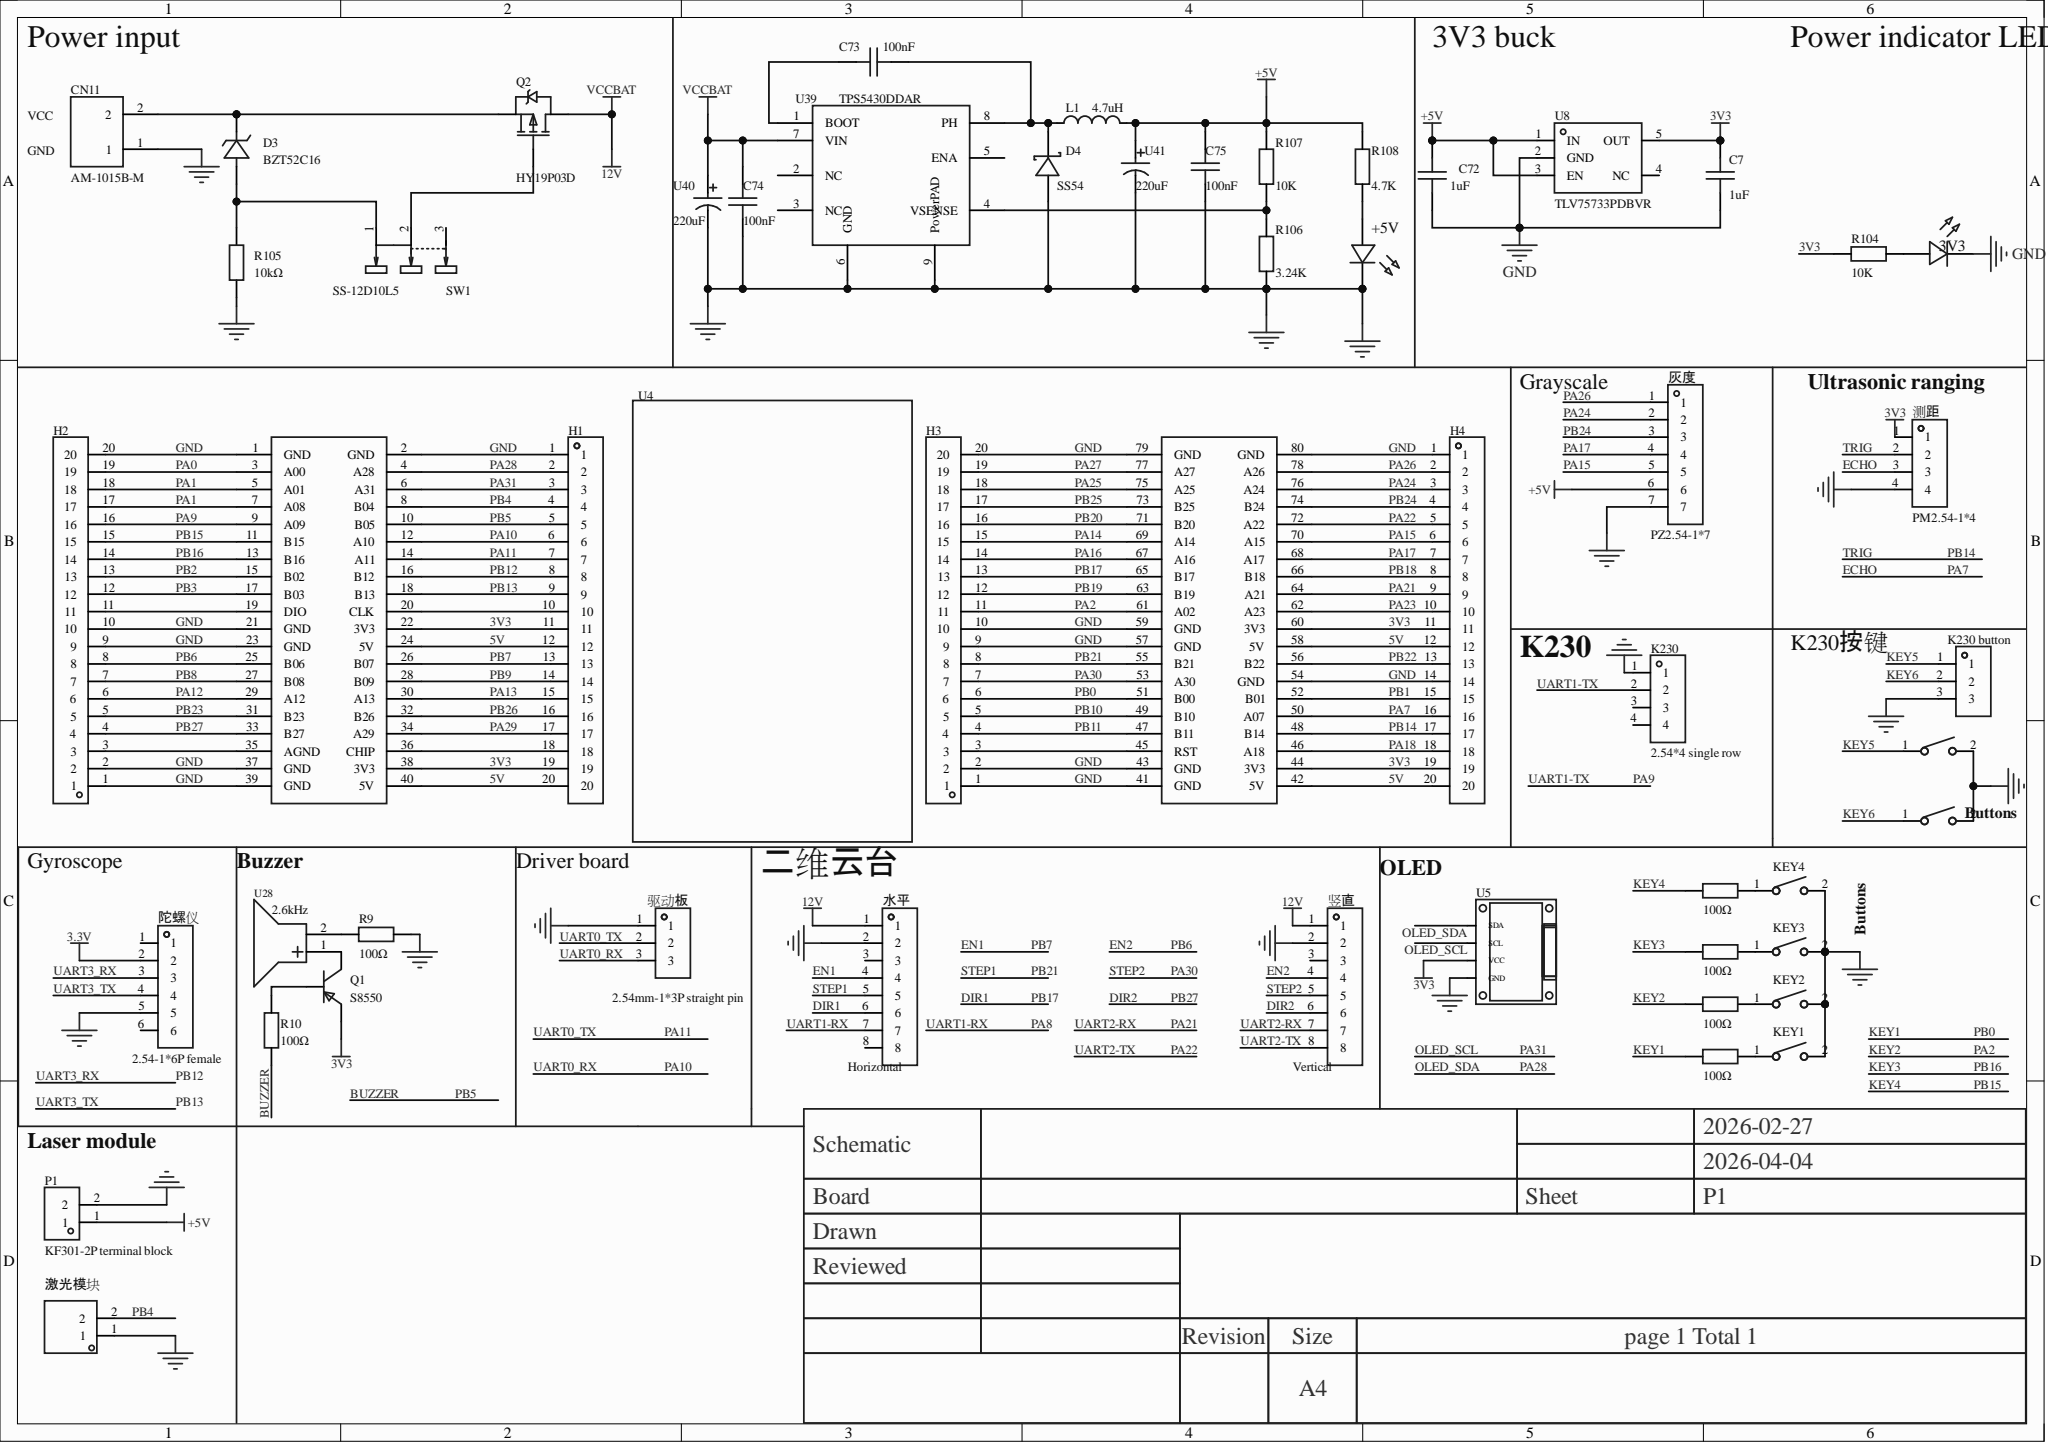Circuit board | Altium Designer | 52 parts | 80 nets
Bill of materials:
Comment,Description,Designator,Footprint,LibRef,Quantity
"","","+5V, 3V3","LED_0603","LED_0603-R","2"
"1uF","","C7, C72","C0603","CAP_0603","2"
"100nF","","C73, C74, C75","C0805","CC0805KRX7R9BB104","3"
"AM-1015B-M","","CN11","CONN-TH_AM-1015B-M","AM-1015B-M","1"
"BZT52C16","","D3","SOD-123_L2.7-W1.6-LS3.7-RD","BZT52C16","1"
"SS54","","D4","SMA_L4.4-W2.8-LS5.4-R-RD","SS54_C22452","1"
"","","H1, H2, H3, H4","HDR-TH_20P-P2.54-V-M-1","HDR-M_2.54_1x20P","4"
"2.54*4 single row","","K230","HDR-TH_4P-P2.54-V-M-1","2.54*4单排","1"
"K230 button","","K230按键","HDR-TH_3P-P2.54-V-M","HDR-M_2.54_1x3P","1"
"Tact switch 3*6*2.5","","K230按键1, K230按键2, KEY1, KEY2, KEY3, KEY4","SW-SMD_L6.0-W3.6-LS8.0","轻触按键3*6*2.5","6"
"4.7uH","","L1","IND-SMD_L7.3-W6.6","MCS0630-4R7MPY1","1"
"KF301-2P terminal block","","P1","CONN-TH_XY301V-A-5.0-2P","KF301-2P接线端子","1"
"S8550","","Q1","SOT-23-3_L2.9-W1.6-P1.90-LS2.8-BR","S8550_C105432","1"
"HY19P03D","","Q2","TO-252-2_L6.6-W6.1-P4.57-LS9.9-TL-CW","HY19P03D","1"
"100Ω","","R9, R10, R109, R110, R111, R112","R0603","Res_0603, 0603WAF1000T5E","6"
"10K","","R104, R107","R0603","Res_0603","2"
"10kΩ","","R105","R0603","0603WAF1002T5E","1"
"3.24K","","R106","R0603","Res_0603","1"
"4.7K","","R108","R0603","Res_0603","1"
"SS-12D10L5","","SW1","SW-TH_SS-12D10L5","SS-12D10L5","1"
"","","U4","COMM-TH_LCKFB-TMX-MSPM0G3507","LCKFB-TMX-MSPM0G3507","1"
"","","U5","0.96OLED_4P","0.96OLED模块_4P","1"
"TLV75733PDBVR","","U8","SOT-23-5_L2.9-W1.6-P0.95-LS2.8-BL","TLV75733PDBVR","1"
"2.6kHz","","U28","BUZ-TH_BD12.0-P7.60-D0.6-FD","HYE1206-05ST","1"
"TPS5430DDAR","","U39","ESOP-8_L4.9-W3.9-P1.27-LS6.0-TL-EP","TPS5430DDAR","1"
"220uF","","U40, U41","CAP-SMD_BD6.3-L6.6-W6.6-LS7.2-FD","220uF","2"
"Horizontal","","水平","CONN-TH_8P-P2.50-XH2.54-8P","XH2.54-8P 直插","1"
"PM2.54-1*4","","测距","HDR-TH_4P-P2.54-V-F","PM2.54-1*4","1"
"","","激光模块","HDR-TH_2P-P2.54-V-M-1","HDR-M_2.54_1x2P","1"
"PZ2.54-1*7","","灰度","HDR-TH_7P-P2.54-V-M","PZ2.54-1*7","1"
"Vertical","","竖直","CONN-TH_8P-P2.50-XH2.54-8P","XH2.54-8P 直插","1"
"2.54-1*6P female","","陀螺仪","HDR-TH_6P-P2.54-V-F","2.54-1*6P母","1"
"2.54mm-1*3P straight pin","","驱动板","HDR-TH_3P-P2.54-V-M-1","2.54mm-1*3P 直针","1"
Netlist (Protel format):
[
3V3
LED_0603




]
[
+5V
LED_0603




]
[
C7
C0603
1uF



]
[
C72
C0603
1uF



]
[
C73
C0805
100nF



]
[
C74
C0805
100nF



]
[
C75
C0805
100nF



]
[
CN11
CONN-TH_AM-1015B-M
AM-1015B-M



]
[
D3
SOD-123_L2.7-W1.6-LS3.7-RD
BZT52C16



]
[
D4
SMA_L4.4-W2.8-LS5.4-R-RD
SS54



]
[
H1
HDR-TH_20P-P2.54-V-M-1




]
[
H2
HDR-TH_20P-P2.54-V-M-1




]
[
H3
HDR-TH_20P-P2.54-V-M-1




]
[
H4
HDR-TH_20P-P2.54-V-M-1




]
[
K230
HDR-TH_4P-P2.54-V-M-1
2.54*4 single row



]
[
K230按键
HDR-TH_3P-P2.54-V-M
K230 button



]
[
K230按键1
SW-SMD_L6.0-W3.6-LS8.0
Tact switch 3*6*2.5



]
[
K230按键2
SW-SMD_L6.0-W3.6-LS8.0
Tact switch 3*6*2.5



]
[
KEY1
SW-SMD_L6.0-W3.6-LS8.0
Tact switch 3*6*2.5



]
[
KEY2
SW-SMD_L6.0-W3.6-LS8.0
Tact switch 3*6*2.5



]
[
KEY3
SW-SMD_L6.0-W3.6-LS8.0
Tact switch 3*6*2.5



]
[
KEY4
SW-SMD_L6.0-W3.6-LS8.0
Tact switch 3*6*2.5



]
[
L1
IND-SMD_L7.3-W6.6
4.7uH



]
[
P1
CONN-TH_XY301V-A-5.0-2P
KF301-2P terminal block



]
[
Q1
SOT-23-3_L2.9-W1.6-P1.90-LS2.8-BR
S8550



]
[
Q2
TO-252-2_L6.6-W6.1-P4.57-LS9.9-TL-CW
HY19P03D



]
[
R9
R0603
100Ω



]
[
R10
R0603
100Ω



]
[
R104
R0603
10K



]
[
R105
R0603
10kΩ



]
[
R106
R0603
3.24K



]
[
R107
R0603
10K



]
[
R108
R0603
4.7K



]
[
R109
R0603
100Ω



]
[
R110
R0603
100Ω



]
[
R111
R0603
100Ω



]
[
R112
R0603
100Ω



]
[
SW1
SW-TH_SS-12D10L5
SS-12D10L5



]
[
U4
COMM-TH_LCKFB-TMX-MSPM0G3507




]
[
U5
0.96OLED_4P




]
[
U8
SOT-23-5_L2.9-W1.6-P0.95-LS2.8-BL
TLV75733PDBVR



]
[
U28
BUZ-TH_BD12.0-P7.60-D0.6-FD
2.6kHz



]
[
U39
ESOP-8_L4.9-W3.9-P1.27-LS6.0-TL-EP
TPS5430DDAR



]
[
U40
CAP-SMD_BD6.3-L6.6-W6.6-LS7.2-FD
220uF



]
[
U41
CAP-SMD_BD6.3-L6.6-W6.6-LS7.2-FD
220uF



]
[
水平
CONN-TH_8P-P2.50-XH2.54-8P
Horizontal



]
[
测距
HDR-TH_4P-P2.54-V-F
PM2.54-1*4



]
[
激光模块
HDR-TH_2P-P2.54-V-M-1




]
[
灰度
HDR-TH_7P-P2.54-V-M
PZ2.54-1*7



]
[
竖直
CONN-TH_8P-P2.50-XH2.54-8P
Vertical



]
[
陀螺仪
HDR-TH_6P-P2.54-V-F
2.54-1*6P female



]
[
驱动板
HDR-TH_3P-P2.54-V-M-1
2.54mm-1*3P straight pin



]
(
PB26
H1-16
U4-32
)
(
PB25
H3-17
U4-73
)
(
PB24
H4-4
U4-74
灰度-3
)
(
PB23
H2-5
U4-31
)
(
PB22
H4-13
U4-56
)
(
PB21
H3-8
U4-55
水平-5
)
(
PB20
H3-16
U4-71
)
(
PB19
H3-12
U4-63
)
(
PB18
H4-8
U4-66
)
(
PB14
H4-17
U4-48
测距-2
)
(
PB13
H1-9
U4-18
陀螺仪-4
)
(
PB12
H1-8
U4-16
陀螺仪-3
)
(
PB11
H3-4
U4-47
)
(
PB10
H3-5
U4-49
)
(
PB9
H1-14
U4-28
)
(
PB8
H2-7
U4-27
)
(
PB4
H1-4
U4-8
激光模块-2
)
(
PB3
H2-12
U4-17
)
(
PB2
H2-13
U4-15
)
(
PB1
H4-15
U4-52
)
(
PA30
H3-7
U4-53
竖直-5
)
(
PA29
H1-17
U4-34
)
(
PA27
H3-19
U4-77
)
(
PA26
H4-2
U4-78
灰度-1
)
(
PA25
H3-18
U4-75
)
(
PA24
H4-3
U4-76
灰度-2
)
(
PA23
H4-10
U4-62
)
(
PA22
H4-5
U4-72
竖直-8
)
(
PA21
H4-9
U4-64
竖直-7
)
(
PA18
H4-18
U4-46
)
(
PA17
H4-7
U4-68
灰度-4
)
(
PA16
H3-14
U4-67
)
(
PA15
H4-6
U4-70
灰度-5
)
(
PA14
H3-15
U4-69
)
(
PA13
H1-15
U4-30
)
(
PA12
H2-6
U4-29
)
(
PA11
H1-7
U4-14
驱动板-2
)
(
PA10
H1-6
U4-12
驱动板-3
)
(
PA9
H2-16
K230-2
U4-9
)
(
PA1
H2-17
H2-18
U4-5
U4-7
)
(
PA0
H2-19
U4-3
)
(
OLED_SDA
H1-2
U4-4
U5-4
)
(
OLED_SCL
H1-3
U4-6
U5-3
)
(
NetR106_2
R106-2
R107-1
U39-4
)
(
NetR9_2
R9-2
U28-2
)
(
NetQ2_1
Q2-1
SW1-2
)
(
NetQ1_3
Q1-3
U28-1
)
(
NetQ1_1
Q1-1
R10-1
)
(
NetKEY4_1
KEY4-1
R112-1
)
(
NetKEY3_1
KEY3-1
R111-1
)
(
NetKEY2_1
KEY2-1
R110-1
)
(
NetKEY1_1
KEY1-1
R109-1
)
(
NetH3_3
H3-3
U4-45
)
(
NetH2_11
H2-11
U4-19
)
(
NetH2_3
H2-3
U4-35
)
(
NetH1_18
H1-18
U4-36
)
(
NetH1_10
H1-10
U4-20
)
(
NetD3_2
D3-2
R105-2
SW1-1
)
(
NetCN11_2
CN11-2
D3-1
Q2-3
)
(
NetC73_2
C73-2
D4-2
L1-1
U39-8
)
(
NetC73_1
C73-1
U39-1
)
(
Net+5V_2
+5V-2
R108-1
)
(
Net3V3_2
3V3-2
R104-2
)
(
KEY6
K230按键-2
K230按键2-1
)
(
KEY5
K230按键-1
K230按键1-1
)
(
KEY4
H2-15
R112-2
U4-11
)
(
KEY3
H2-14
R111-2
U4-13
)
(
KEY2
H3-11
R110-2
U4-61
)
(
KEY1
H3-6
R109-2
U4-51
)
(
GND
3V3-1
+5V-1
C7-1
C72-1
C74-1
C75-1
CN11-1
D4-1
H1-1
H2-1
H2-2
H2-9
H2-10
H2-20
H3-1
H3-2
H3-9
H3-10
H3-20
H4-1
H4-14
K230-1
K230按键-3
K230按键1-2
K230按键2-2
KEY1-2
KEY2-2
KEY3-2
KEY4-2
P1-2
R9-1
R105-1
R106-1
U4-1
U4-2
U4-21
U4-23
U4-37
U4-39
U4-41
U4-43
U4-54
U4-57
U4-59
U4-79
U4-80
U5-1
U8-2
U39-6
U39-9
U40-2
U41-2
水平-2
测距-4
激光模块-1
灰度-7
竖直-2
陀螺仪-5
驱动板-1
)
(
EN2
H2-8
U4-25
竖直-4
)
(
EN1
H1-13
U4-26
水平-4
)
(
ECHO
H4-16
U4-50
测距-3
)
(
DIR2
H2-4
U4-33
竖直-6
)
(
DIR1
H3-13
U4-65
水平-6
)
(
BUZZER
H1-5
R10-2
U4-10
)
(
+5V
C72-2
C75-2
L1-2
P1-1
R107-2
R108-2
U8-1
U8-3
U41-1
灰度-6
)
(
12V
C74-2
Q2-2
U39-7
U40-1
水平-1
竖直-1
)
(
5V
H1-12
H1-20
H4-12
H4-20
U4-24
U4-40
U4-42
U4-58
)
(
3V3
C7-2
H1-11
H1-19
H4-11
H4-19
Q1-2
R104-1
U4-22
U4-38
U4-44
U4-60
U5-2
U8-5
测距-1
)